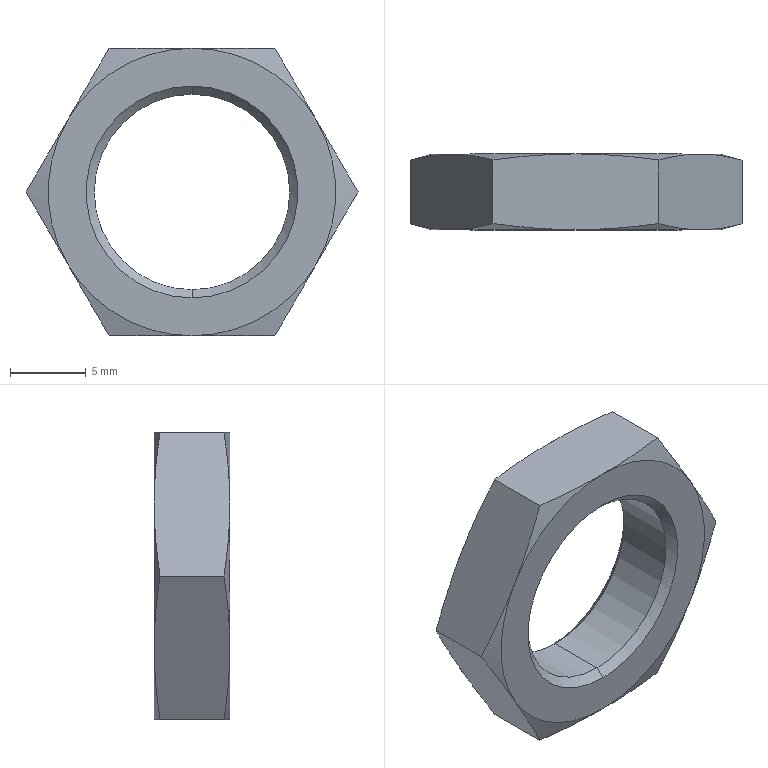Part | SolidWorks | features RefAxis 3, 3DProfileFeature 1, ICE 1, Revolution 1 | 1 solid | 26 faces | box 21.939 x 5 x 19 mm | volume 888.805 mm3 | cone 16 | plane 8 | cylinder 2 | commonest cylinder face diameters 12.917 x2
STEP:
#1=CARTESIAN_POINT('',(0.,1.958,-6.458));
#2=VERTEX_POINT('',#1);
#3=CARTESIAN_POINT('',(0.,1.958,6.458));
#4=VERTEX_POINT('',#3);
#5=CARTESIAN_POINT('',(0.,1.958,0.));
#6=DIRECTION('',(0.,1.,0.));
#7=DIRECTION('',(0.,0.,1.));
#8=AXIS2_PLACEMENT_3D('',#5,#6,#7);
#9=CIRCLE('',#8,6.458);
#10=EDGE_CURVE('',#2,#4,#9,.T.);
#11=ORIENTED_EDGE('',*,*,#10,.F.);
#12=CARTESIAN_POINT('',(0.,2.5,-7.));
#13=VERTEX_POINT('',#12);
#14=CARTESIAN_POINT('',(0.,2.5,-7.));
#15=DIRECTION('',(0.,0.7071,-0.7071));
#16=VECTOR('',#15,1000.);
#17=LINE('',#14,#16);
#18=EDGE_CURVE('',#2,#13,#17,.T.);
#19=ORIENTED_EDGE('',*,*,#18,.T.);
#20=CARTESIAN_POINT('',(0.,2.5,7.));
#21=VERTEX_POINT('',#20);
#22=CARTESIAN_POINT('',(0.,2.5,0.));
#23=DIRECTION('',(0.,1.,0.));
#24=DIRECTION('',(0.,0.,1.));
#25=AXIS2_PLACEMENT_3D('',#22,#23,#24);
#26=CIRCLE('',#25,7.);
#27=EDGE_CURVE('',#13,#21,#26,.T.);
#28=ORIENTED_EDGE('',*,*,#27,.T.);
#29=CARTESIAN_POINT('',(0.,2.5,7.));
#30=DIRECTION('',(0.,0.7071,0.7071));
#31=VECTOR('',#30,1000.);
#32=LINE('',#29,#31);
#33=EDGE_CURVE('',#4,#21,#32,.T.);
#34=ORIENTED_EDGE('',*,*,#33,.F.);
#35=EDGE_LOOP('',(#11,#19,#28,#34));
#36=FACE_OUTER_BOUND('',#35,.T.);
#37=CARTESIAN_POINT('',(0.,2.5,0.));
#38=DIRECTION('',(0.,1.,0.));
#39=DIRECTION('',(0.,0.,1.));
#40=AXIS2_PLACEMENT_3D('',#37,#38,#39);
#41=CONICAL_SURFACE('',#40,7.,0.7854);
#42=ADVANCED_FACE('',(#36),#41,.F.);
#43=CARTESIAN_POINT('',(0.,-1.958,-6.458));
#44=VERTEX_POINT('',#43);
#45=CARTESIAN_POINT('',(0.,-1.958,6.458));
#46=VERTEX_POINT('',#45);
#47=CARTESIAN_POINT('',(0.,-1.958,0.));
#48=DIRECTION('',(0.,1.,0.));
#49=DIRECTION('',(0.,0.,1.));
#50=AXIS2_PLACEMENT_3D('',#47,#48,#49);
#51=CIRCLE('',#50,6.458);
#52=EDGE_CURVE('',#44,#46,#51,.T.);
#53=ORIENTED_EDGE('',*,*,#52,.T.);
#54=CARTESIAN_POINT('',(0.,-2.5,7.));
#55=VERTEX_POINT('',#54);
#56=CARTESIAN_POINT('',(0.,-1.958,6.458));
#57=DIRECTION('',(0.,-0.7071,0.7071));
#58=VECTOR('',#57,1000.);
#59=LINE('',#56,#58);
#60=EDGE_CURVE('',#46,#55,#59,.T.);
#61=ORIENTED_EDGE('',*,*,#60,.T.);
#62=CARTESIAN_POINT('',(0.,-2.5,-7.));
#63=VERTEX_POINT('',#62);
#64=CARTESIAN_POINT('',(0.,-2.5,0.));
#65=DIRECTION('',(0.,1.,0.));
#66=DIRECTION('',(0.,0.,1.));
#67=AXIS2_PLACEMENT_3D('',#64,#65,#66);
#68=CIRCLE('',#67,7.);
#69=EDGE_CURVE('',#63,#55,#68,.T.);
#70=ORIENTED_EDGE('',*,*,#69,.F.);
#71=CARTESIAN_POINT('',(0.,-1.958,-6.458));
#72=DIRECTION('',(0.,-0.7071,-0.7071));
#73=VECTOR('',#72,1000.);
#74=LINE('',#71,#73);
#75=EDGE_CURVE('',#44,#63,#74,.T.);
#76=ORIENTED_EDGE('',*,*,#75,.F.);
#77=EDGE_LOOP('',(#53,#61,#70,#76));
#78=FACE_OUTER_BOUND('',#77,.T.);
#79=CARTESIAN_POINT('',(0.,-1.958,0.));
#80=DIRECTION('',(0.,-1.,0.));
#81=DIRECTION('',(0.,0.,-1.));
#82=AXIS2_PLACEMENT_3D('',#79,#80,#81);
#83=CONICAL_SURFACE('',#82,6.458,0.7854);
#84=ADVANCED_FACE('',(#78),#83,.F.);
#85=ORIENTED_EDGE('',*,*,#52,.F.);
#86=CARTESIAN_POINT('',(0.,-2.5,-6.458));
#87=DIRECTION('',(0.,1.,0.));
#88=VECTOR('',#87,1000.);
#89=LINE('',#86,#88);
#90=EDGE_CURVE('',#44,#2,#89,.T.);
#91=ORIENTED_EDGE('',*,*,#90,.T.);
#92=ORIENTED_EDGE('',*,*,#10,.T.);
#93=CARTESIAN_POINT('',(0.,-2.5,6.458));
#94=DIRECTION('',(0.,1.,0.));
#95=VECTOR('',#94,1000.);
#96=LINE('',#93,#95);
#97=EDGE_CURVE('',#46,#4,#96,.T.);
#98=ORIENTED_EDGE('',*,*,#97,.F.);
#99=EDGE_LOOP('',(#85,#91,#92,#98));
#100=FACE_OUTER_BOUND('',#99,.T.);
#101=CARTESIAN_POINT('',(0.,-2.5,0.));
#102=DIRECTION('',(0.,1.,0.));
#103=DIRECTION('',(0.,0.,1.));
#104=AXIS2_PLACEMENT_3D('',#101,#102,#103);
#105=CYLINDRICAL_SURFACE('',#104,6.458);
#106=ADVANCED_FACE('',(#100),#105,.F.);
#107=CARTESIAN_POINT('',(10.97,-2.106,0.));
#108=VERTEX_POINT('',#107);
#109=CARTESIAN_POINT('',(8.227,-2.5,-4.75));
#110=VERTEX_POINT('',#109);
#111=CARTESIAN_POINT('',(10.97,-2.106,0.));
#112=CARTESIAN_POINT('',(10.513,-2.229,-0.7917));
#113=CARTESIAN_POINT('',(10.056,-2.328,-1.583));
#114=CARTESIAN_POINT('',(9.141,-2.464,-3.167));
#115=CARTESIAN_POINT('',(8.684,-2.5,-3.958));
#116=CARTESIAN_POINT('',(8.227,-2.5,-4.75));
#117=B_SPLINE_CURVE_WITH_KNOTS('',3,(#111,#112,#113,#114,#115,#116),.UNSPECIFIED.,.F.,.F.,(4,2,4),(0.000000231,0.002743,0.005485),.UNSPECIFIED.);
#118=EDGE_CURVE('',#108,#110,#117,.T.);
#119=ORIENTED_EDGE('',*,*,#118,.F.);
#120=CARTESIAN_POINT('',(8.227,-2.5,4.75));
#121=VERTEX_POINT('',#120);
#122=CARTESIAN_POINT('',(8.227,-2.5,4.75));
#123=CARTESIAN_POINT('',(8.684,-2.5,3.958));
#124=CARTESIAN_POINT('',(9.141,-2.464,3.167));
#125=CARTESIAN_POINT('',(10.056,-2.328,1.583));
#126=CARTESIAN_POINT('',(10.513,-2.229,0.7917));
#127=CARTESIAN_POINT('',(10.97,-2.106,0.));
#128=B_SPLINE_CURVE_WITH_KNOTS('',3,(#122,#123,#124,#125,#126,#127),.UNSPECIFIED.,.F.,.F.,(4,2,4),(0.005485,0.008227,0.01097),.UNSPECIFIED.);
#129=EDGE_CURVE('',#121,#108,#128,.T.);
#130=ORIENTED_EDGE('',*,*,#129,.F.);
#131=CARTESIAN_POINT('',(0.,-2.5,0.));
#132=DIRECTION('',(0.,1.,0.));
#133=DIRECTION('',(0.,0.,1.));
#134=AXIS2_PLACEMENT_3D('',#131,#132,#133);
#135=CIRCLE('',#134,9.5);
#136=EDGE_CURVE('',#121,#110,#135,.T.);
#137=ORIENTED_EDGE('',*,*,#136,.T.);
#138=EDGE_LOOP('',(#119,#130,#137));
#139=FACE_OUTER_BOUND('',#138,.T.);
#140=CARTESIAN_POINT('',(0.,-2.5,0.));
#141=DIRECTION('',(0.,1.,0.));
#142=DIRECTION('',(0.,0.,1.));
#143=AXIS2_PLACEMENT_3D('',#140,#141,#142);
#144=CONICAL_SURFACE('',#143,9.5,1.309);
#145=ADVANCED_FACE('',(#139),#144,.T.);
#146=CARTESIAN_POINT('',(5.485,-2.106,-9.5));
#147=VERTEX_POINT('',#146);
#148=CARTESIAN_POINT('',(8.227,-2.5,-4.75));
#149=CARTESIAN_POINT('',(7.77,-2.5,-5.542));
#150=CARTESIAN_POINT('',(7.313,-2.464,-6.333));
#151=CARTESIAN_POINT('',(6.399,-2.328,-7.917));
#152=CARTESIAN_POINT('',(5.942,-2.229,-8.708));
#153=CARTESIAN_POINT('',(5.485,-2.106,-9.5));
#154=B_SPLINE_CURVE_WITH_KNOTS('',3,(#148,#149,#150,#151,#152,#153),.UNSPECIFIED.,.F.,.F.,(4,2,4),(0.005485,0.008227,0.01097),.UNSPECIFIED.);
#155=EDGE_CURVE('',#110,#147,#154,.T.);
#156=ORIENTED_EDGE('',*,*,#155,.F.);
#157=CARTESIAN_POINT('',(0.,-2.5,-9.5));
#158=VERTEX_POINT('',#157);
#159=CARTESIAN_POINT('',(0.,-2.5,0.));
#160=DIRECTION('',(0.,1.,0.));
#161=DIRECTION('',(0.,0.,1.));
#162=AXIS2_PLACEMENT_3D('',#159,#160,#161);
#163=CIRCLE('',#162,9.5);
#164=EDGE_CURVE('',#110,#158,#163,.T.);
#165=ORIENTED_EDGE('',*,*,#164,.T.);
#166=CARTESIAN_POINT('',(5.485,-2.106,-9.5));
#167=CARTESIAN_POINT('',(4.572,-2.228,-9.5));
#168=CARTESIAN_POINT('',(3.659,-2.328,-9.5));
#169=CARTESIAN_POINT('',(1.831,-2.464,-9.5));
#170=CARTESIAN_POINT('',(0.916,-2.5,-9.5));
#171=CARTESIAN_POINT('',(0.,-2.5,-9.5));
#172=B_SPLINE_CURVE_WITH_KNOTS('',3,(#166,#167,#168,#169,#170,#171),.UNSPECIFIED.,.F.,.F.,(4,2,4),(0.02129,0.02405,0.02681),.UNSPECIFIED.);
#173=EDGE_CURVE('',#147,#158,#172,.T.);
#174=ORIENTED_EDGE('',*,*,#173,.F.);
#175=EDGE_LOOP('',(#156,#165,#174));
#176=FACE_OUTER_BOUND('',#175,.T.);
#177=CARTESIAN_POINT('',(0.,-2.5,0.));
#178=DIRECTION('',(0.,1.,0.));
#179=DIRECTION('',(0.,0.,1.));
#180=AXIS2_PLACEMENT_3D('',#177,#178,#179);
#181=CONICAL_SURFACE('',#180,9.5,1.309);
#182=ADVANCED_FACE('',(#176),#181,.T.);
#183=CARTESIAN_POINT('',(-5.485,-2.106,-9.5));
#184=VERTEX_POINT('',#183);
#185=CARTESIAN_POINT('',(0.,-2.5,-9.5));
#186=CARTESIAN_POINT('',(-0.9129,-2.5,-9.5));
#187=CARTESIAN_POINT('',(-1.827,-2.464,-9.5));
#188=CARTESIAN_POINT('',(-3.656,-2.328,-9.5));
#189=CARTESIAN_POINT('',(-4.573,-2.228,-9.5));
#190=CARTESIAN_POINT('',(-5.485,-2.106,-9.5));
#191=B_SPLINE_CURVE_WITH_KNOTS('',3,(#185,#186,#187,#188,#189,#190),.UNSPECIFIED.,.F.,.F.,(4,2,4),(0.02681,0.02956,0.03231),.UNSPECIFIED.);
#192=EDGE_CURVE('',#158,#184,#191,.T.);
#193=ORIENTED_EDGE('',*,*,#192,.F.);
#194=CARTESIAN_POINT('',(-8.227,-2.5,-4.75));
#195=VERTEX_POINT('',#194);
#196=CARTESIAN_POINT('',(0.,-2.5,0.));
#197=DIRECTION('',(0.,1.,0.));
#198=DIRECTION('',(0.,0.,1.));
#199=AXIS2_PLACEMENT_3D('',#196,#197,#198);
#200=CIRCLE('',#199,9.5);
#201=EDGE_CURVE('',#158,#195,#200,.T.);
#202=ORIENTED_EDGE('',*,*,#201,.T.);
#203=CARTESIAN_POINT('',(-5.485,-2.106,-9.5));
#204=CARTESIAN_POINT('',(-5.942,-2.229,-8.708));
#205=CARTESIAN_POINT('',(-6.399,-2.328,-7.917));
#206=CARTESIAN_POINT('',(-7.313,-2.464,-6.333));
#207=CARTESIAN_POINT('',(-7.77,-2.5,-5.542));
#208=CARTESIAN_POINT('',(-8.227,-2.5,-4.75));
#209=B_SPLINE_CURVE_WITH_KNOTS('',3,(#203,#204,#205,#206,#207,#208),.UNSPECIFIED.,.F.,.F.,(4,2,4),(0.000000231,0.002743,0.005485),.UNSPECIFIED.);
#210=EDGE_CURVE('',#184,#195,#209,.T.);
#211=ORIENTED_EDGE('',*,*,#210,.F.);
#212=EDGE_LOOP('',(#193,#202,#211));
#213=FACE_OUTER_BOUND('',#212,.T.);
#214=CARTESIAN_POINT('',(0.,-2.5,0.));
#215=DIRECTION('',(0.,1.,0.));
#216=DIRECTION('',(0.,0.,1.));
#217=AXIS2_PLACEMENT_3D('',#214,#215,#216);
#218=CONICAL_SURFACE('',#217,9.5,1.309);
#219=ADVANCED_FACE('',(#213),#218,.T.);
#220=CARTESIAN_POINT('',(5.485,-2.106,9.5));
#221=VERTEX_POINT('',#220);
#222=CARTESIAN_POINT('',(5.485,-2.106,9.5));
#223=CARTESIAN_POINT('',(5.942,-2.229,8.708));
#224=CARTESIAN_POINT('',(6.399,-2.328,7.917));
#225=CARTESIAN_POINT('',(7.313,-2.464,6.333));
#226=CARTESIAN_POINT('',(7.77,-2.5,5.542));
#227=CARTESIAN_POINT('',(8.227,-2.5,4.75));
#228=B_SPLINE_CURVE_WITH_KNOTS('',3,(#222,#223,#224,#225,#226,#227),.UNSPECIFIED.,.F.,.F.,(4,2,4),(0.000000231,0.002743,0.005485),.UNSPECIFIED.);
#229=EDGE_CURVE('',#221,#121,#228,.T.);
#230=ORIENTED_EDGE('',*,*,#229,.F.);
#231=CARTESIAN_POINT('',(0.,-2.5,9.5));
#232=VERTEX_POINT('',#231);
#233=CARTESIAN_POINT('',(0.,-2.5,9.5));
#234=CARTESIAN_POINT('',(0.916,-2.5,9.5));
#235=CARTESIAN_POINT('',(1.831,-2.464,9.5));
#236=CARTESIAN_POINT('',(3.659,-2.328,9.5));
#237=CARTESIAN_POINT('',(4.572,-2.228,9.5));
#238=CARTESIAN_POINT('',(5.485,-2.106,9.5));
#239=B_SPLINE_CURVE_WITH_KNOTS('',3,(#233,#234,#235,#236,#237,#238),.UNSPECIFIED.,.F.,.F.,(4,2,4),(0.01477,0.01753,0.0203),.UNSPECIFIED.);
#240=EDGE_CURVE('',#232,#221,#239,.T.);
#241=ORIENTED_EDGE('',*,*,#240,.F.);
#242=CARTESIAN_POINT('',(0.,-2.5,0.));
#243=DIRECTION('',(0.,1.,0.));
#244=DIRECTION('',(0.,0.,1.));
#245=AXIS2_PLACEMENT_3D('',#242,#243,#244);
#246=CIRCLE('',#245,9.5);
#247=EDGE_CURVE('',#232,#121,#246,.T.);
#248=ORIENTED_EDGE('',*,*,#247,.T.);
#249=EDGE_LOOP('',(#230,#241,#248));
#250=FACE_OUTER_BOUND('',#249,.T.);
#251=CARTESIAN_POINT('',(0.,-2.5,0.));
#252=DIRECTION('',(0.,1.,0.));
#253=DIRECTION('',(0.,0.,1.));
#254=AXIS2_PLACEMENT_3D('',#251,#252,#253);
#255=CONICAL_SURFACE('',#254,9.5,1.309);
#256=ADVANCED_FACE('',(#250),#255,.T.);
#257=CARTESIAN_POINT('',(-10.97,-2.106,0.));
#258=VERTEX_POINT('',#257);
#259=CARTESIAN_POINT('',(-8.227,-2.5,-4.75));
#260=CARTESIAN_POINT('',(-8.684,-2.5,-3.958));
#261=CARTESIAN_POINT('',(-9.141,-2.464,-3.167));
#262=CARTESIAN_POINT('',(-10.056,-2.328,-1.583));
#263=CARTESIAN_POINT('',(-10.513,-2.229,-0.7917));
#264=CARTESIAN_POINT('',(-10.97,-2.106,0.));
#265=B_SPLINE_CURVE_WITH_KNOTS('',3,(#259,#260,#261,#262,#263,#264),.UNSPECIFIED.,.F.,.F.,(4,2,4),(0.005485,0.008227,0.01097),.UNSPECIFIED.);
#266=EDGE_CURVE('',#195,#258,#265,.T.);
#267=ORIENTED_EDGE('',*,*,#266,.F.);
#268=CARTESIAN_POINT('',(-8.227,-2.5,4.75));
#269=VERTEX_POINT('',#268);
#270=CARTESIAN_POINT('',(0.,-2.5,0.));
#271=DIRECTION('',(0.,1.,0.));
#272=DIRECTION('',(0.,0.,1.));
#273=AXIS2_PLACEMENT_3D('',#270,#271,#272);
#274=CIRCLE('',#273,9.5);
#275=EDGE_CURVE('',#195,#269,#274,.T.);
#276=ORIENTED_EDGE('',*,*,#275,.T.);
#277=CARTESIAN_POINT('',(-10.97,-2.106,0.));
#278=CARTESIAN_POINT('',(-10.513,-2.229,0.7917));
#279=CARTESIAN_POINT('',(-10.056,-2.328,1.583));
#280=CARTESIAN_POINT('',(-9.141,-2.464,3.167));
#281=CARTESIAN_POINT('',(-8.684,-2.5,3.958));
#282=CARTESIAN_POINT('',(-8.227,-2.5,4.75));
#283=B_SPLINE_CURVE_WITH_KNOTS('',3,(#277,#278,#279,#280,#281,#282),.UNSPECIFIED.,.F.,.F.,(4,2,4),(0.000000231,0.002743,0.005485),.UNSPECIFIED.);
#284=EDGE_CURVE('',#258,#269,#283,.T.);
#285=ORIENTED_EDGE('',*,*,#284,.F.);
#286=EDGE_LOOP('',(#267,#276,#285));
#287=FACE_OUTER_BOUND('',#286,.T.);
#288=CARTESIAN_POINT('',(0.,-2.5,0.));
#289=DIRECTION('',(0.,1.,0.));
#290=DIRECTION('',(0.,0.,1.));
#291=AXIS2_PLACEMENT_3D('',#288,#289,#290);
#292=CONICAL_SURFACE('',#291,9.5,1.309);
#293=ADVANCED_FACE('',(#287),#292,.T.);
#294=CARTESIAN_POINT('',(-5.485,-2.106,9.5));
#295=VERTEX_POINT('',#294);
#296=CARTESIAN_POINT('',(-5.485,-2.106,9.5));
#297=CARTESIAN_POINT('',(-4.573,-2.228,9.5));
#298=CARTESIAN_POINT('',(-3.656,-2.328,9.5));
#299=CARTESIAN_POINT('',(-1.827,-2.464,9.5));
#300=CARTESIAN_POINT('',(-0.9129,-2.5,9.5));
#301=CARTESIAN_POINT('',(0.,-2.5,9.5));
#302=B_SPLINE_CURVE_WITH_KNOTS('',3,(#296,#297,#298,#299,#300,#301),.UNSPECIFIED.,.F.,.F.,(4,2,4),(0.009256,0.01201,0.01477),.UNSPECIFIED.);
#303=EDGE_CURVE('',#295,#232,#302,.T.);
#304=ORIENTED_EDGE('',*,*,#303,.F.);
#305=CARTESIAN_POINT('',(-8.227,-2.5,4.75));
#306=CARTESIAN_POINT('',(-7.77,-2.5,5.542));
#307=CARTESIAN_POINT('',(-7.313,-2.464,6.333));
#308=CARTESIAN_POINT('',(-6.399,-2.328,7.917));
#309=CARTESIAN_POINT('',(-5.942,-2.229,8.708));
#310=CARTESIAN_POINT('',(-5.485,-2.106,9.5));
#311=B_SPLINE_CURVE_WITH_KNOTS('',3,(#305,#306,#307,#308,#309,#310),.UNSPECIFIED.,.F.,.F.,(4,2,4),(0.005485,0.008227,0.01097),.UNSPECIFIED.);
#312=EDGE_CURVE('',#269,#295,#311,.T.);
#313=ORIENTED_EDGE('',*,*,#312,.F.);
#314=CARTESIAN_POINT('',(0.,-2.5,0.));
#315=DIRECTION('',(0.,1.,0.));
#316=DIRECTION('',(0.,0.,1.));
#317=AXIS2_PLACEMENT_3D('',#314,#315,#316);
#318=CIRCLE('',#317,9.5);
#319=EDGE_CURVE('',#269,#232,#318,.T.);
#320=ORIENTED_EDGE('',*,*,#319,.T.);
#321=EDGE_LOOP('',(#304,#313,#320));
#322=FACE_OUTER_BOUND('',#321,.T.);
#323=CARTESIAN_POINT('',(0.,-2.5,0.));
#324=DIRECTION('',(0.,1.,0.));
#325=DIRECTION('',(0.,0.,1.));
#326=AXIS2_PLACEMENT_3D('',#323,#324,#325);
#327=CONICAL_SURFACE('',#326,9.5,1.309);
#328=ADVANCED_FACE('',(#322),#327,.T.);
#329=CARTESIAN_POINT('',(-10.97,2.106,0.));
#330=VERTEX_POINT('',#329);
#331=CARTESIAN_POINT('',(-8.227,2.5,-4.75));
#332=VERTEX_POINT('',#331);
#333=CARTESIAN_POINT('',(-10.97,2.106,0.));
#334=CARTESIAN_POINT('',(-10.513,2.229,-0.7917));
#335=CARTESIAN_POINT('',(-10.056,2.328,-1.583));
#336=CARTESIAN_POINT('',(-9.141,2.464,-3.167));
#337=CARTESIAN_POINT('',(-8.684,2.5,-3.958));
#338=CARTESIAN_POINT('',(-8.227,2.5,-4.75));
#339=B_SPLINE_CURVE_WITH_KNOTS('',3,(#333,#334,#335,#336,#337,#338),.UNSPECIFIED.,.F.,.F.,(4,2,4),(0.000000231,0.002743,0.005485),.UNSPECIFIED.);
#340=EDGE_CURVE('',#330,#332,#339,.T.);
#341=ORIENTED_EDGE('',*,*,#340,.F.);
#342=CARTESIAN_POINT('',(-8.227,2.5,4.75));
#343=VERTEX_POINT('',#342);
#344=CARTESIAN_POINT('',(-8.227,2.5,4.75));
#345=CARTESIAN_POINT('',(-8.684,2.5,3.958));
#346=CARTESIAN_POINT('',(-9.141,2.464,3.167));
#347=CARTESIAN_POINT('',(-10.056,2.328,1.583));
#348=CARTESIAN_POINT('',(-10.513,2.229,0.7917));
#349=CARTESIAN_POINT('',(-10.97,2.106,0.));
#350=B_SPLINE_CURVE_WITH_KNOTS('',3,(#344,#345,#346,#347,#348,#349),.UNSPECIFIED.,.F.,.F.,(4,2,4),(0.005485,0.008227,0.01097),.UNSPECIFIED.);
#351=EDGE_CURVE('',#343,#330,#350,.T.);
#352=ORIENTED_EDGE('',*,*,#351,.F.);
#353=CARTESIAN_POINT('',(0.,2.5,0.));
#354=DIRECTION('',(0.,1.,0.));
#355=DIRECTION('',(0.,0.,1.));
#356=AXIS2_PLACEMENT_3D('',#353,#354,#355);
#357=CIRCLE('',#356,9.5);
#358=EDGE_CURVE('',#332,#343,#357,.T.);
#359=ORIENTED_EDGE('',*,*,#358,.F.);
#360=EDGE_LOOP('',(#341,#352,#359));
#361=FACE_OUTER_BOUND('',#360,.T.);
#362=CARTESIAN_POINT('',(0.,1.026,0.));
#363=DIRECTION('',(0.,-1.,0.));
#364=DIRECTION('',(0.,0.,-1.));
#365=AXIS2_PLACEMENT_3D('',#362,#363,#364);
#366=CONICAL_SURFACE('',#365,15.,1.309);
#367=ADVANCED_FACE('',(#361),#366,.T.);
#368=CARTESIAN_POINT('',(-5.485,2.106,-9.5));
#369=VERTEX_POINT('',#368);
#370=CARTESIAN_POINT('',(-8.227,2.5,-4.75));
#371=CARTESIAN_POINT('',(-7.77,2.5,-5.542));
#372=CARTESIAN_POINT('',(-7.313,2.464,-6.333));
#373=CARTESIAN_POINT('',(-6.399,2.328,-7.917));
#374=CARTESIAN_POINT('',(-5.942,2.229,-8.708));
#375=CARTESIAN_POINT('',(-5.485,2.106,-9.5));
#376=B_SPLINE_CURVE_WITH_KNOTS('',3,(#370,#371,#372,#373,#374,#375),.UNSPECIFIED.,.F.,.F.,(4,2,4),(0.005485,0.008227,0.01097),.UNSPECIFIED.);
#377=EDGE_CURVE('',#332,#369,#376,.T.);
#378=ORIENTED_EDGE('',*,*,#377,.F.);
#379=CARTESIAN_POINT('',(0.,2.5,-9.5));
#380=VERTEX_POINT('',#379);
#381=CARTESIAN_POINT('',(0.,2.5,0.));
#382=DIRECTION('',(0.,1.,0.));
#383=DIRECTION('',(0.,0.,1.));
#384=AXIS2_PLACEMENT_3D('',#381,#382,#383);
#385=CIRCLE('',#384,9.5);
#386=EDGE_CURVE('',#380,#332,#385,.T.);
#387=ORIENTED_EDGE('',*,*,#386,.F.);
#388=CARTESIAN_POINT('',(-5.485,2.106,-9.5));
#389=CARTESIAN_POINT('',(-4.573,2.228,-9.5));
#390=CARTESIAN_POINT('',(-3.656,2.328,-9.5));
#391=CARTESIAN_POINT('',(-1.827,2.464,-9.5));
#392=CARTESIAN_POINT('',(-0.9129,2.5,-9.5));
#393=CARTESIAN_POINT('',(0.,2.5,-9.5));
#394=B_SPLINE_CURVE_WITH_KNOTS('',3,(#388,#389,#390,#391,#392,#393),.UNSPECIFIED.,.F.,.F.,(4,2,4),(0.009256,0.01201,0.01477),.UNSPECIFIED.);
#395=EDGE_CURVE('',#369,#380,#394,.T.);
#396=ORIENTED_EDGE('',*,*,#395,.F.);
#397=EDGE_LOOP('',(#378,#387,#396));
#398=FACE_OUTER_BOUND('',#397,.T.);
#399=CARTESIAN_POINT('',(0.,1.026,0.));
#400=DIRECTION('',(0.,-1.,0.));
#401=DIRECTION('',(0.,0.,-1.));
#402=AXIS2_PLACEMENT_3D('',#399,#400,#401);
#403=CONICAL_SURFACE('',#402,15.,1.309);
#404=ADVANCED_FACE('',(#398),#403,.T.);
#405=CARTESIAN_POINT('',(5.485,2.106,-9.5));
#406=VERTEX_POINT('',#405);
#407=CARTESIAN_POINT('',(0.,2.5,-9.5));
#408=CARTESIAN_POINT('',(0.916,2.5,-9.5));
#409=CARTESIAN_POINT('',(1.831,2.464,-9.5));
#410=CARTESIAN_POINT('',(3.659,2.328,-9.5));
#411=CARTESIAN_POINT('',(4.572,2.228,-9.5));
#412=CARTESIAN_POINT('',(5.485,2.106,-9.5));
#413=B_SPLINE_CURVE_WITH_KNOTS('',3,(#407,#408,#409,#410,#411,#412),.UNSPECIFIED.,.F.,.F.,(4,2,4),(0.01477,0.01753,0.0203),.UNSPECIFIED.);
#414=EDGE_CURVE('',#380,#406,#413,.T.);
#415=ORIENTED_EDGE('',*,*,#414,.F.);
#416=CARTESIAN_POINT('',(8.227,2.5,-4.75));
#417=VERTEX_POINT('',#416);
#418=CARTESIAN_POINT('',(0.,2.5,0.));
#419=DIRECTION('',(0.,1.,0.));
#420=DIRECTION('',(0.,0.,1.));
#421=AXIS2_PLACEMENT_3D('',#418,#419,#420);
#422=CIRCLE('',#421,9.5);
#423=EDGE_CURVE('',#417,#380,#422,.T.);
#424=ORIENTED_EDGE('',*,*,#423,.F.);
#425=CARTESIAN_POINT('',(5.485,2.106,-9.5));
#426=CARTESIAN_POINT('',(5.942,2.229,-8.708));
#427=CARTESIAN_POINT('',(6.399,2.328,-7.917));
#428=CARTESIAN_POINT('',(7.313,2.464,-6.333));
#429=CARTESIAN_POINT('',(7.77,2.5,-5.542));
#430=CARTESIAN_POINT('',(8.227,2.5,-4.75));
#431=B_SPLINE_CURVE_WITH_KNOTS('',3,(#425,#426,#427,#428,#429,#430),.UNSPECIFIED.,.F.,.F.,(4,2,4),(0.000000231,0.002743,0.005485),.UNSPECIFIED.);
#432=EDGE_CURVE('',#406,#417,#431,.T.);
#433=ORIENTED_EDGE('',*,*,#432,.F.);
#434=EDGE_LOOP('',(#415,#424,#433));
#435=FACE_OUTER_BOUND('',#434,.T.);
#436=CARTESIAN_POINT('',(0.,1.026,0.));
#437=DIRECTION('',(0.,-1.,0.));
#438=DIRECTION('',(0.,0.,-1.));
#439=AXIS2_PLACEMENT_3D('',#436,#437,#438);
#440=CONICAL_SURFACE('',#439,15.,1.309);
#441=ADVANCED_FACE('',(#435),#440,.T.);
#442=CARTESIAN_POINT('',(10.97,2.106,0.));
#443=VERTEX_POINT('',#442);
#444=CARTESIAN_POINT('',(8.227,2.5,-4.75));
#445=CARTESIAN_POINT('',(8.684,2.5,-3.958));
#446=CARTESIAN_POINT('',(9.141,2.464,-3.167));
#447=CARTESIAN_POINT('',(10.056,2.328,-1.583));
#448=CARTESIAN_POINT('',(10.513,2.229,-0.7917));
#449=CARTESIAN_POINT('',(10.97,2.106,0.));
#450=B_SPLINE_CURVE_WITH_KNOTS('',3,(#444,#445,#446,#447,#448,#449),.UNSPECIFIED.,.F.,.F.,(4,2,4),(0.005485,0.008227,0.01097),.UNSPECIFIED.);
#451=EDGE_CURVE('',#417,#443,#450,.T.);
#452=ORIENTED_EDGE('',*,*,#451,.F.);
#453=CARTESIAN_POINT('',(8.227,2.5,4.75));
#454=VERTEX_POINT('',#453);
#455=CARTESIAN_POINT('',(0.,2.5,0.));
#456=DIRECTION('',(0.,1.,0.));
#457=DIRECTION('',(0.,0.,1.));
#458=AXIS2_PLACEMENT_3D('',#455,#456,#457);
#459=CIRCLE('',#458,9.5);
#460=EDGE_CURVE('',#454,#417,#459,.T.);
#461=ORIENTED_EDGE('',*,*,#460,.F.);
#462=CARTESIAN_POINT('',(10.97,2.106,0.));
#463=CARTESIAN_POINT('',(10.513,2.229,0.7917));
#464=CARTESIAN_POINT('',(10.056,2.328,1.583));
#465=CARTESIAN_POINT('',(9.141,2.464,3.167));
#466=CARTESIAN_POINT('',(8.684,2.5,3.958));
#467=CARTESIAN_POINT('',(8.227,2.5,4.75));
#468=B_SPLINE_CURVE_WITH_KNOTS('',3,(#462,#463,#464,#465,#466,#467),.UNSPECIFIED.,.F.,.F.,(4,2,4),(0.000000231,0.002743,0.005485),.UNSPECIFIED.);
#469=EDGE_CURVE('',#443,#454,#468,.T.);
#470=ORIENTED_EDGE('',*,*,#469,.F.);
#471=EDGE_LOOP('',(#452,#461,#470));
#472=FACE_OUTER_BOUND('',#471,.T.);
#473=CARTESIAN_POINT('',(0.,1.026,0.));
#474=DIRECTION('',(0.,-1.,0.));
#475=DIRECTION('',(0.,0.,-1.));
#476=AXIS2_PLACEMENT_3D('',#473,#474,#475);
#477=CONICAL_SURFACE('',#476,15.,1.309);
#478=ADVANCED_FACE('',(#472),#477,.T.);
#479=CARTESIAN_POINT('',(5.485,2.106,9.5));
#480=VERTEX_POINT('',#479);
#481=CARTESIAN_POINT('',(8.227,2.5,4.75));
#482=CARTESIAN_POINT('',(7.77,2.5,5.542));
#483=CARTESIAN_POINT('',(7.313,2.464,6.333));
#484=CARTESIAN_POINT('',(6.399,2.328,7.917));
#485=CARTESIAN_POINT('',(5.942,2.229,8.708));
#486=CARTESIAN_POINT('',(5.485,2.106,9.5));
#487=B_SPLINE_CURVE_WITH_KNOTS('',3,(#481,#482,#483,#484,#485,#486),.UNSPECIFIED.,.F.,.F.,(4,2,4),(0.005485,0.008227,0.01097),.UNSPECIFIED.);
#488=EDGE_CURVE('',#454,#480,#487,.T.);
#489=ORIENTED_EDGE('',*,*,#488,.F.);
#490=CARTESIAN_POINT('',(0.,2.5,9.5));
#491=VERTEX_POINT('',#490);
#492=CARTESIAN_POINT('',(0.,2.5,0.));
#493=DIRECTION('',(0.,1.,0.));
#494=DIRECTION('',(0.,0.,1.));
#495=AXIS2_PLACEMENT_3D('',#492,#493,#494);
#496=CIRCLE('',#495,9.5);
#497=EDGE_CURVE('',#491,#454,#496,.T.);
#498=ORIENTED_EDGE('',*,*,#497,.F.);
#499=CARTESIAN_POINT('',(5.485,2.106,9.5));
#500=CARTESIAN_POINT('',(4.572,2.228,9.5));
#501=CARTESIAN_POINT('',(3.659,2.328,9.5));
#502=CARTESIAN_POINT('',(1.831,2.464,9.5));
#503=CARTESIAN_POINT('',(0.916,2.5,9.5));
#504=CARTESIAN_POINT('',(0.,2.5,9.5));
#505=B_SPLINE_CURVE_WITH_KNOTS('',3,(#499,#500,#501,#502,#503,#504),.UNSPECIFIED.,.F.,.F.,(4,2,4),(0.02129,0.02405,0.02681),.UNSPECIFIED.);
#506=EDGE_CURVE('',#480,#491,#505,.T.);
#507=ORIENTED_EDGE('',*,*,#506,.F.);
#508=EDGE_LOOP('',(#489,#498,#507));
#509=FACE_OUTER_BOUND('',#508,.T.);
#510=CARTESIAN_POINT('',(0.,1.026,0.));
#511=DIRECTION('',(0.,-1.,0.));
#512=DIRECTION('',(0.,0.,-1.));
#513=AXIS2_PLACEMENT_3D('',#510,#511,#512);
#514=CONICAL_SURFACE('',#513,15.,1.309);
#515=ADVANCED_FACE('',(#509),#514,.T.);
#516=CARTESIAN_POINT('',(-5.485,2.106,9.5));
#517=VERTEX_POINT('',#516);
#518=CARTESIAN_POINT('',(0.,2.5,9.5));
#519=CARTESIAN_POINT('',(-0.9129,2.5,9.5));
#520=CARTESIAN_POINT('',(-1.827,2.464,9.5));
#521=CARTESIAN_POINT('',(-3.656,2.328,9.5));
#522=CARTESIAN_POINT('',(-4.573,2.228,9.5));
#523=CARTESIAN_POINT('',(-5.485,2.106,9.5));
#524=B_SPLINE_CURVE_WITH_KNOTS('',3,(#518,#519,#520,#521,#522,#523),.UNSPECIFIED.,.F.,.F.,(4,2,4),(0.02681,0.02956,0.03231),.UNSPECIFIED.);
#525=EDGE_CURVE('',#491,#517,#524,.T.);
#526=ORIENTED_EDGE('',*,*,#525,.F.);
#527=CARTESIAN_POINT('',(0.,2.5,0.));
#528=DIRECTION('',(0.,1.,0.));
#529=DIRECTION('',(0.,0.,1.));
#530=AXIS2_PLACEMENT_3D('',#527,#528,#529);
#531=CIRCLE('',#530,9.5);
#532=EDGE_CURVE('',#343,#491,#531,.T.);
#533=ORIENTED_EDGE('',*,*,#532,.F.);
#534=CARTESIAN_POINT('',(-5.485,2.106,9.5));
#535=CARTESIAN_POINT('',(-5.942,2.229,8.708));
#536=CARTESIAN_POINT('',(-6.399,2.328,7.917));
#537=CARTESIAN_POINT('',(-7.313,2.464,6.333));
#538=CARTESIAN_POINT('',(-7.77,2.5,5.542));
#539=CARTESIAN_POINT('',(-8.227,2.5,4.75));
#540=B_SPLINE_CURVE_WITH_KNOTS('',3,(#534,#535,#536,#537,#538,#539),.UNSPECIFIED.,.F.,.F.,(4,2,4),(0.000000231,0.002743,0.005485),.UNSPECIFIED.);
#541=EDGE_CURVE('',#517,#343,#540,.T.);
#542=ORIENTED_EDGE('',*,*,#541,.F.);
#543=EDGE_LOOP('',(#526,#533,#542));
#544=FACE_OUTER_BOUND('',#543,.T.);
#545=CARTESIAN_POINT('',(0.,1.026,0.));
#546=DIRECTION('',(0.,-1.,0.));
#547=DIRECTION('',(0.,0.,-1.));
#548=AXIS2_PLACEMENT_3D('',#545,#546,#547);
#549=CONICAL_SURFACE('',#548,15.,1.309);
#550=ADVANCED_FACE('',(#544),#549,.T.);
#551=ORIENTED_EDGE('',*,*,#90,.F.);
#552=CARTESIAN_POINT('',(0.,-1.958,0.));
#553=DIRECTION('',(0.,1.,0.));
#554=DIRECTION('',(0.,0.,1.));
#555=AXIS2_PLACEMENT_3D('',#552,#553,#554);
#556=CIRCLE('',#555,6.458);
#557=EDGE_CURVE('',#46,#44,#556,.T.);
#558=ORIENTED_EDGE('',*,*,#557,.F.);
#559=ORIENTED_EDGE('',*,*,#97,.T.);
#560=CARTESIAN_POINT('',(0.,1.958,0.));
#561=DIRECTION('',(0.,1.,0.));
#562=DIRECTION('',(0.,0.,1.));
#563=AXIS2_PLACEMENT_3D('',#560,#561,#562);
#564=CIRCLE('',#563,6.458);
#565=EDGE_CURVE('',#4,#2,#564,.T.);
#566=ORIENTED_EDGE('',*,*,#565,.T.);
#567=EDGE_LOOP('',(#551,#558,#559,#566));
#568=FACE_OUTER_BOUND('',#567,.T.);
#569=CARTESIAN_POINT('',(0.,-2.5,0.));
#570=DIRECTION('',(0.,1.,0.));
#571=DIRECTION('',(0.,0.,1.));
#572=AXIS2_PLACEMENT_3D('',#569,#570,#571);
#573=CYLINDRICAL_SURFACE('',#572,6.458);
#574=ADVANCED_FACE('',(#568),#573,.F.);
#575=ORIENTED_EDGE('',*,*,#60,.F.);
#576=ORIENTED_EDGE('',*,*,#557,.T.);
#577=ORIENTED_EDGE('',*,*,#75,.T.);
#578=CARTESIAN_POINT('',(0.,-2.5,0.));
#579=DIRECTION('',(0.,1.,0.));
#580=DIRECTION('',(0.,0.,1.));
#581=AXIS2_PLACEMENT_3D('',#578,#579,#580);
#582=CIRCLE('',#581,7.);
#583=EDGE_CURVE('',#55,#63,#582,.T.);
#584=ORIENTED_EDGE('',*,*,#583,.F.);
#585=EDGE_LOOP('',(#575,#576,#577,#584));
#586=FACE_OUTER_BOUND('',#585,.T.);
#587=CARTESIAN_POINT('',(0.,-1.958,0.));
#588=DIRECTION('',(0.,-1.,0.));
#589=DIRECTION('',(0.,0.,-1.));
#590=AXIS2_PLACEMENT_3D('',#587,#588,#589);
#591=CONICAL_SURFACE('',#590,6.458,0.7854);
#592=ADVANCED_FACE('',(#586),#591,.F.);
#593=ORIENTED_EDGE('',*,*,#247,.F.);
#594=ORIENTED_EDGE('',*,*,#319,.F.);
#595=ORIENTED_EDGE('',*,*,#275,.F.);
#596=ORIENTED_EDGE('',*,*,#201,.F.);
#597=ORIENTED_EDGE('',*,*,#164,.F.);
#598=ORIENTED_EDGE('',*,*,#136,.F.);
#599=EDGE_LOOP('',(#593,#594,#595,#596,#597,#598));
#600=FACE_OUTER_BOUND('',#599,.T.);
#601=ORIENTED_EDGE('',*,*,#69,.T.);
#602=ORIENTED_EDGE('',*,*,#583,.T.);
#603=EDGE_LOOP('',(#601,#602));
#604=FACE_BOUND('',#603,.T.);
#605=CARTESIAN_POINT('',(7.,-2.5,0.));
#606=DIRECTION('',(0.,1.,0.));
#607=DIRECTION('',(0.,0.,1.));
#608=AXIS2_PLACEMENT_3D('',#605,#606,#607);
#609=PLANE('',#608);
#610=ADVANCED_FACE('',(#600,#604),#609,.F.);
#611=CARTESIAN_POINT('',(0.,2.5,0.));
#612=DIRECTION('',(0.,1.,0.));
#613=DIRECTION('',(0.,0.,1.));
#614=AXIS2_PLACEMENT_3D('',#611,#612,#613);
#615=CIRCLE('',#614,7.);
#616=EDGE_CURVE('',#21,#13,#615,.T.);
#617=ORIENTED_EDGE('',*,*,#616,.F.);
#618=ORIENTED_EDGE('',*,*,#27,.F.);
#619=EDGE_LOOP('',(#617,#618));
#620=FACE_BOUND('',#619,.T.);
#621=ORIENTED_EDGE('',*,*,#497,.T.);
#622=ORIENTED_EDGE('',*,*,#460,.T.);
#623=ORIENTED_EDGE('',*,*,#423,.T.);
#624=ORIENTED_EDGE('',*,*,#386,.T.);
#625=ORIENTED_EDGE('',*,*,#358,.T.);
#626=ORIENTED_EDGE('',*,*,#532,.T.);
#627=EDGE_LOOP('',(#621,#622,#623,#624,#625,#626));
#628=FACE_OUTER_BOUND('',#627,.T.);
#629=CARTESIAN_POINT('',(9.5,2.5,0.));
#630=DIRECTION('',(0.,-1.,0.));
#631=DIRECTION('',(0.,0.,-1.));
#632=AXIS2_PLACEMENT_3D('',#629,#630,#631);
#633=PLANE('',#632);
#634=ADVANCED_FACE('',(#620,#628),#633,.F.);
#635=ORIENTED_EDGE('',*,*,#18,.F.);
#636=ORIENTED_EDGE('',*,*,#565,.F.);
#637=ORIENTED_EDGE('',*,*,#33,.T.);
#638=ORIENTED_EDGE('',*,*,#616,.T.);
#639=EDGE_LOOP('',(#635,#636,#637,#638));
#640=FACE_OUTER_BOUND('',#639,.T.);
#641=CARTESIAN_POINT('',(0.,2.5,0.));
#642=DIRECTION('',(0.,1.,0.));
#643=DIRECTION('',(0.,0.,1.));
#644=AXIS2_PLACEMENT_3D('',#641,#642,#643);
#645=CONICAL_SURFACE('',#644,7.,0.7854);
#646=ADVANCED_FACE('',(#640),#645,.F.);
#647=ORIENTED_EDGE('',*,*,#210,.T.);
#648=ORIENTED_EDGE('',*,*,#266,.T.);
#649=CARTESIAN_POINT('',(-10.97,-2.5,0.));
#650=DIRECTION('',(0.,1.,0.));
#651=VECTOR('',#650,1000.);
#652=LINE('',#649,#651);
#653=EDGE_CURVE('',#258,#330,#652,.T.);
#654=ORIENTED_EDGE('',*,*,#653,.T.);
#655=ORIENTED_EDGE('',*,*,#340,.T.);
#656=ORIENTED_EDGE('',*,*,#377,.T.);
#657=CARTESIAN_POINT('',(-5.485,-2.5,-9.5));
#658=DIRECTION('',(0.,1.,0.));
#659=VECTOR('',#658,1000.);
#660=LINE('',#657,#659);
#661=EDGE_CURVE('',#184,#369,#660,.T.);
#662=ORIENTED_EDGE('',*,*,#661,.F.);
#663=EDGE_LOOP('',(#647,#648,#654,#655,#656,#662));
#664=FACE_OUTER_BOUND('',#663,.T.);
#665=CARTESIAN_POINT('',(-5.485,-2.5,-9.5));
#666=DIRECTION('',(-0.866,0.,-0.5));
#667=DIRECTION('',(-0.5,0.,0.866));
#668=AXIS2_PLACEMENT_3D('',#665,#666,#667);
#669=PLANE('',#668);
#670=ADVANCED_FACE('',(#664),#669,.T.);
#671=ORIENTED_EDGE('',*,*,#173,.T.);
#672=ORIENTED_EDGE('',*,*,#192,.T.);
#673=ORIENTED_EDGE('',*,*,#661,.T.);
#674=ORIENTED_EDGE('',*,*,#395,.T.);
#675=ORIENTED_EDGE('',*,*,#414,.T.);
#676=CARTESIAN_POINT('',(5.485,-2.5,-9.5));
#677=DIRECTION('',(0.,1.,0.));
#678=VECTOR('',#677,1000.);
#679=LINE('',#676,#678);
#680=EDGE_CURVE('',#147,#406,#679,.T.);
#681=ORIENTED_EDGE('',*,*,#680,.F.);
#682=EDGE_LOOP('',(#671,#672,#673,#674,#675,#681));
#683=FACE_OUTER_BOUND('',#682,.T.);
#684=CARTESIAN_POINT('',(5.485,-2.5,-9.5));
#685=DIRECTION('',(0.,0.,-1.));
#686=DIRECTION('',(-1.,0.,0.));
#687=AXIS2_PLACEMENT_3D('',#684,#685,#686);
#688=PLANE('',#687);
#689=ADVANCED_FACE('',(#683),#688,.T.);
#690=ORIENTED_EDGE('',*,*,#118,.T.);
#691=ORIENTED_EDGE('',*,*,#155,.T.);
#692=ORIENTED_EDGE('',*,*,#680,.T.);
#693=ORIENTED_EDGE('',*,*,#432,.T.);
#694=ORIENTED_EDGE('',*,*,#451,.T.);
#695=CARTESIAN_POINT('',(10.97,-2.5,0.));
#696=DIRECTION('',(0.,1.,0.));
#697=VECTOR('',#696,1000.);
#698=LINE('',#695,#697);
#699=EDGE_CURVE('',#108,#443,#698,.T.);
#700=ORIENTED_EDGE('',*,*,#699,.F.);
#701=EDGE_LOOP('',(#690,#691,#692,#693,#694,#700));
#702=FACE_OUTER_BOUND('',#701,.T.);
#703=CARTESIAN_POINT('',(10.97,-2.5,0.));
#704=DIRECTION('',(0.866,0.,-0.5));
#705=DIRECTION('',(-0.5,0.,-0.866));
#706=AXIS2_PLACEMENT_3D('',#703,#704,#705);
#707=PLANE('',#706);
#708=ADVANCED_FACE('',(#702),#707,.T.);
#709=ORIENTED_EDGE('',*,*,#229,.T.);
#710=ORIENTED_EDGE('',*,*,#129,.T.);
#711=ORIENTED_EDGE('',*,*,#699,.T.);
#712=ORIENTED_EDGE('',*,*,#469,.T.);
#713=ORIENTED_EDGE('',*,*,#488,.T.);
#714=CARTESIAN_POINT('',(5.485,-2.5,9.5));
#715=DIRECTION('',(0.,1.,0.));
#716=VECTOR('',#715,1000.);
#717=LINE('',#714,#716);
#718=EDGE_CURVE('',#221,#480,#717,.T.);
#719=ORIENTED_EDGE('',*,*,#718,.F.);
#720=EDGE_LOOP('',(#709,#710,#711,#712,#713,#719));
#721=FACE_OUTER_BOUND('',#720,.T.);
#722=CARTESIAN_POINT('',(5.485,-2.5,9.5));
#723=DIRECTION('',(0.866,0.,0.5));
#724=DIRECTION('',(0.5,0.,-0.866));
#725=AXIS2_PLACEMENT_3D('',#722,#723,#724);
#726=PLANE('',#725);
#727=ADVANCED_FACE('',(#721),#726,.T.);
#728=ORIENTED_EDGE('',*,*,#303,.T.);
#729=ORIENTED_EDGE('',*,*,#240,.T.);
#730=ORIENTED_EDGE('',*,*,#718,.T.);
#731=ORIENTED_EDGE('',*,*,#506,.T.);
#732=ORIENTED_EDGE('',*,*,#525,.T.);
#733=CARTESIAN_POINT('',(-5.485,-2.5,9.5));
#734=DIRECTION('',(0.,1.,0.));
#735=VECTOR('',#734,1000.);
#736=LINE('',#733,#735);
#737=EDGE_CURVE('',#295,#517,#736,.T.);
#738=ORIENTED_EDGE('',*,*,#737,.F.);
#739=EDGE_LOOP('',(#728,#729,#730,#731,#732,#738));
#740=FACE_OUTER_BOUND('',#739,.T.);
#741=CARTESIAN_POINT('',(-5.485,-2.5,9.5));
#742=DIRECTION('',(0.,0.,1.));
#743=DIRECTION('',(1.,0.,0.));
#744=AXIS2_PLACEMENT_3D('',#741,#742,#743);
#745=PLANE('',#744);
#746=ADVANCED_FACE('',(#740),#745,.T.);
#747=ORIENTED_EDGE('',*,*,#284,.T.);
#748=ORIENTED_EDGE('',*,*,#312,.T.);
#749=ORIENTED_EDGE('',*,*,#737,.T.);
#750=ORIENTED_EDGE('',*,*,#541,.T.);
#751=ORIENTED_EDGE('',*,*,#351,.T.);
#752=ORIENTED_EDGE('',*,*,#653,.F.);
#753=EDGE_LOOP('',(#747,#748,#749,#750,#751,#752));
#754=FACE_OUTER_BOUND('',#753,.T.);
#755=CARTESIAN_POINT('',(-10.97,-2.5,0.));
#756=DIRECTION('',(-0.866,0.,0.5));
#757=DIRECTION('',(0.5,0.,0.866));
#758=AXIS2_PLACEMENT_3D('',#755,#756,#757);
#759=PLANE('',#758);
#760=ADVANCED_FACE('',(#754),#759,.T.);
#761=CLOSED_SHELL('',(#42,#84,#106,#145,#182,#219,#256,#293,#328,#367,#404,#441,#478,#515,#550,#574,#592,#610,#634,#646,#670,#689,#708,#727,#746,#760));
#762=MANIFOLD_SOLID_BREP('',#761);
#763=CARTESIAN_POINT('',(0.,0.,0.));
#764=DIRECTION('',(0.,0.,1.));
#765=DIRECTION('',(1.,0.,0.));
#766=AXIS2_PLACEMENT_3D('',#763,#764,#765);
#767=(LENGTH_UNIT()NAMED_UNIT(*)SI_UNIT(.MILLI.,.METRE.));
#768=UNCERTAINTY_MEASURE_WITH_UNIT(LENGTH_MEASURE(0.00001),#767,'','');
#769=(NAMED_UNIT(*)PLANE_ANGLE_UNIT()SI_UNIT($,.RADIAN.));
#770=(NAMED_UNIT(*)SI_UNIT($,.STERADIAN.)SOLID_ANGLE_UNIT());
#771=(GEOMETRIC_REPRESENTATION_CONTEXT(3)GLOBAL_UNCERTAINTY_ASSIGNED_CONTEXT((#768))GLOBAL_UNIT_ASSIGNED_CONTEXT((#767,#769,#770))REPRESENTATION_CONTEXT('',''));
#772=ADVANCED_BREP_SHAPE_REPRESENTATION('',(#762,#766),#771);